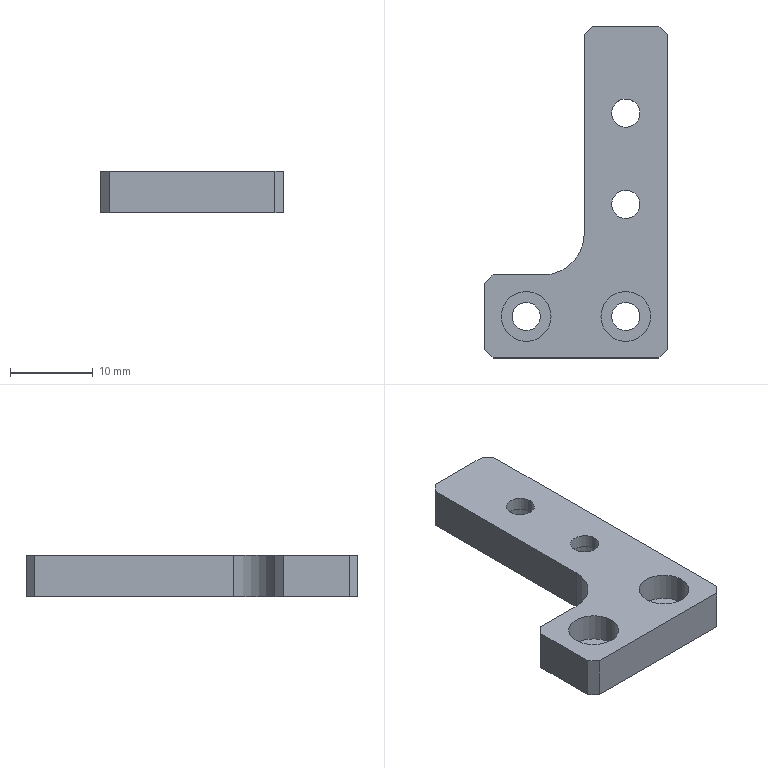Part | STEP file | FBDS-TL-003 | 1 solid | 34 faces | box 22 x 40 x 5 mm | volume 2172 mm3 | cylinder 17 | plane 17 | commonest cylinder face diameters 3.4 x8 6 x8 10 x1
STEP:
#1=CARTESIAN_POINT('',(-3.,-15.,1.6));
#2=VERTEX_POINT('',#1);
#3=CARTESIAN_POINT('',(3.,-15.,1.6));
#4=VERTEX_POINT('',#3);
#5=CARTESIAN_POINT('',(0.,-15.,1.6));
#6=DIRECTION('',(0.,0.,1.));
#7=DIRECTION('',(1.,0.,0.));
#8=AXIS2_PLACEMENT_3D('',#5,#6,#7);
#9=CIRCLE('',#8,3.);
#10=EDGE_CURVE('',#2,#4,#9,.T.);
#11=ORIENTED_EDGE('',*,*,#10,.F.);
#12=CARTESIAN_POINT('',(-3.,-15.,5.));
#13=VERTEX_POINT('',#12);
#14=CARTESIAN_POINT('',(-3.,-15.,5.));
#15=DIRECTION('',(0.,0.,1.));
#16=VECTOR('',#15,1000.);
#17=LINE('',#14,#16);
#18=EDGE_CURVE('',#2,#13,#17,.T.);
#19=ORIENTED_EDGE('',*,*,#18,.T.);
#20=CARTESIAN_POINT('',(3.,-15.,5.));
#21=VERTEX_POINT('',#20);
#22=CARTESIAN_POINT('',(0.,-15.,5.));
#23=DIRECTION('',(0.,0.,1.));
#24=DIRECTION('',(1.,0.,0.));
#25=AXIS2_PLACEMENT_3D('',#22,#23,#24);
#26=CIRCLE('',#25,3.);
#27=EDGE_CURVE('',#13,#21,#26,.T.);
#28=ORIENTED_EDGE('',*,*,#27,.T.);
#29=CARTESIAN_POINT('',(3.,-15.,5.));
#30=DIRECTION('',(0.,0.,1.));
#31=VECTOR('',#30,1000.);
#32=LINE('',#29,#31);
#33=EDGE_CURVE('',#4,#21,#32,.T.);
#34=ORIENTED_EDGE('',*,*,#33,.F.);
#35=EDGE_LOOP('',(#11,#19,#28,#34));
#36=FACE_OUTER_BOUND('',#35,.T.);
#37=CARTESIAN_POINT('',(0.,-15.,5.));
#38=DIRECTION('',(0.,0.,1.));
#39=DIRECTION('',(1.,0.,0.));
#40=AXIS2_PLACEMENT_3D('',#37,#38,#39);
#41=CYLINDRICAL_SURFACE('',#40,3.);
#42=ADVANCED_FACE('',(#36),#41,.F.);
#43=CARTESIAN_POINT('',(1.7,-15.,0.));
#44=VERTEX_POINT('',#43);
#45=CARTESIAN_POINT('',(-1.7,-15.,0.));
#46=VERTEX_POINT('',#45);
#47=CARTESIAN_POINT('',(0.,-15.,0.));
#48=DIRECTION('',(0.,0.,-1.));
#49=DIRECTION('',(-1.,0.,0.));
#50=AXIS2_PLACEMENT_3D('',#47,#48,#49);
#51=CIRCLE('',#50,1.7);
#52=EDGE_CURVE('',#44,#46,#51,.T.);
#53=ORIENTED_EDGE('',*,*,#52,.T.);
#54=CARTESIAN_POINT('',(-1.7,-15.,1.6));
#55=VERTEX_POINT('',#54);
#56=CARTESIAN_POINT('',(-1.7,-15.,5.));
#57=DIRECTION('',(0.,0.,1.));
#58=VECTOR('',#57,1000.);
#59=LINE('',#56,#58);
#60=EDGE_CURVE('',#46,#55,#59,.T.);
#61=ORIENTED_EDGE('',*,*,#60,.T.);
#62=CARTESIAN_POINT('',(1.7,-15.,1.6));
#63=VERTEX_POINT('',#62);
#64=CARTESIAN_POINT('',(0.,-15.,1.6));
#65=DIRECTION('',(0.,0.,1.));
#66=DIRECTION('',(1.,0.,0.));
#67=AXIS2_PLACEMENT_3D('',#64,#65,#66);
#68=CIRCLE('',#67,1.7);
#69=EDGE_CURVE('',#55,#63,#68,.T.);
#70=ORIENTED_EDGE('',*,*,#69,.T.);
#71=CARTESIAN_POINT('',(1.7,-15.,5.));
#72=DIRECTION('',(0.,0.,1.));
#73=VECTOR('',#72,1000.);
#74=LINE('',#71,#73);
#75=EDGE_CURVE('',#44,#63,#74,.T.);
#76=ORIENTED_EDGE('',*,*,#75,.F.);
#77=EDGE_LOOP('',(#53,#61,#70,#76));
#78=FACE_OUTER_BOUND('',#77,.T.);
#79=CARTESIAN_POINT('',(0.,-15.,5.));
#80=DIRECTION('',(0.,0.,1.));
#81=DIRECTION('',(1.,0.,0.));
#82=AXIS2_PLACEMENT_3D('',#79,#80,#81);
#83=CYLINDRICAL_SURFACE('',#82,1.7);
#84=ADVANCED_FACE('',(#78),#83,.F.);
#85=CARTESIAN_POINT('',(-15.,-15.,1.6));
#86=VERTEX_POINT('',#85);
#87=CARTESIAN_POINT('',(-9.,-15.,1.6));
#88=VERTEX_POINT('',#87);
#89=CARTESIAN_POINT('',(-12.,-15.,1.6));
#90=DIRECTION('',(0.,0.,1.));
#91=DIRECTION('',(1.,0.,0.));
#92=AXIS2_PLACEMENT_3D('',#89,#90,#91);
#93=CIRCLE('',#92,3.);
#94=EDGE_CURVE('',#86,#88,#93,.T.);
#95=ORIENTED_EDGE('',*,*,#94,.F.);
#96=CARTESIAN_POINT('',(-15.,-15.,5.));
#97=VERTEX_POINT('',#96);
#98=CARTESIAN_POINT('',(-15.,-15.,5.));
#99=DIRECTION('',(0.,0.,1.));
#100=VECTOR('',#99,1000.);
#101=LINE('',#98,#100);
#102=EDGE_CURVE('',#86,#97,#101,.T.);
#103=ORIENTED_EDGE('',*,*,#102,.T.);
#104=CARTESIAN_POINT('',(-9.,-15.,5.));
#105=VERTEX_POINT('',#104);
#106=CARTESIAN_POINT('',(-12.,-15.,5.));
#107=DIRECTION('',(0.,0.,1.));
#108=DIRECTION('',(1.,0.,0.));
#109=AXIS2_PLACEMENT_3D('',#106,#107,#108);
#110=CIRCLE('',#109,3.);
#111=EDGE_CURVE('',#97,#105,#110,.T.);
#112=ORIENTED_EDGE('',*,*,#111,.T.);
#113=CARTESIAN_POINT('',(-9.,-15.,5.));
#114=DIRECTION('',(0.,0.,1.));
#115=VECTOR('',#114,1000.);
#116=LINE('',#113,#115);
#117=EDGE_CURVE('',#88,#105,#116,.T.);
#118=ORIENTED_EDGE('',*,*,#117,.F.);
#119=EDGE_LOOP('',(#95,#103,#112,#118));
#120=FACE_OUTER_BOUND('',#119,.T.);
#121=CARTESIAN_POINT('',(-12.,-15.,5.));
#122=DIRECTION('',(0.,0.,1.));
#123=DIRECTION('',(1.,0.,0.));
#124=AXIS2_PLACEMENT_3D('',#121,#122,#123);
#125=CYLINDRICAL_SURFACE('',#124,3.);
#126=ADVANCED_FACE('',(#120),#125,.F.);
#127=CARTESIAN_POINT('',(-10.3,-15.,0.));
#128=VERTEX_POINT('',#127);
#129=CARTESIAN_POINT('',(-13.7,-15.,0.));
#130=VERTEX_POINT('',#129);
#131=CARTESIAN_POINT('',(-12.,-15.,0.));
#132=DIRECTION('',(0.,0.,-1.));
#133=DIRECTION('',(-1.,0.,0.));
#134=AXIS2_PLACEMENT_3D('',#131,#132,#133);
#135=CIRCLE('',#134,1.7);
#136=EDGE_CURVE('',#128,#130,#135,.T.);
#137=ORIENTED_EDGE('',*,*,#136,.T.);
#138=CARTESIAN_POINT('',(-13.7,-15.,1.6));
#139=VERTEX_POINT('',#138);
#140=CARTESIAN_POINT('',(-13.7,-15.,5.));
#141=DIRECTION('',(0.,0.,1.));
#142=VECTOR('',#141,1000.);
#143=LINE('',#140,#142);
#144=EDGE_CURVE('',#130,#139,#143,.T.);
#145=ORIENTED_EDGE('',*,*,#144,.T.);
#146=CARTESIAN_POINT('',(-10.3,-15.,1.6));
#147=VERTEX_POINT('',#146);
#148=CARTESIAN_POINT('',(-12.,-15.,1.6));
#149=DIRECTION('',(0.,0.,1.));
#150=DIRECTION('',(1.,0.,0.));
#151=AXIS2_PLACEMENT_3D('',#148,#149,#150);
#152=CIRCLE('',#151,1.7);
#153=EDGE_CURVE('',#139,#147,#152,.T.);
#154=ORIENTED_EDGE('',*,*,#153,.T.);
#155=CARTESIAN_POINT('',(-10.3,-15.,5.));
#156=DIRECTION('',(0.,0.,1.));
#157=VECTOR('',#156,1000.);
#158=LINE('',#155,#157);
#159=EDGE_CURVE('',#128,#147,#158,.T.);
#160=ORIENTED_EDGE('',*,*,#159,.F.);
#161=EDGE_LOOP('',(#137,#145,#154,#160));
#162=FACE_OUTER_BOUND('',#161,.T.);
#163=CARTESIAN_POINT('',(-12.,-15.,5.));
#164=DIRECTION('',(0.,0.,1.));
#165=DIRECTION('',(1.,0.,0.));
#166=AXIS2_PLACEMENT_3D('',#163,#164,#165);
#167=CYLINDRICAL_SURFACE('',#166,1.7);
#168=ADVANCED_FACE('',(#162),#167,.F.);
#169=CARTESIAN_POINT('',(3.,-1.5,3.4));
#170=VERTEX_POINT('',#169);
#171=CARTESIAN_POINT('',(-3.,-1.5,3.4));
#172=VERTEX_POINT('',#171);
#173=CARTESIAN_POINT('',(0.,-1.5,3.4));
#174=DIRECTION('',(0.,0.,-1.));
#175=DIRECTION('',(-1.,0.,0.));
#176=AXIS2_PLACEMENT_3D('',#173,#174,#175);
#177=CIRCLE('',#176,3.);
#178=EDGE_CURVE('',#170,#172,#177,.T.);
#179=ORIENTED_EDGE('',*,*,#178,.F.);
#180=CARTESIAN_POINT('',(3.,-1.5,0.));
#181=VERTEX_POINT('',#180);
#182=CARTESIAN_POINT('',(3.,-1.5,0.));
#183=DIRECTION('',(0.,0.,-1.));
#184=VECTOR('',#183,1000.);
#185=LINE('',#182,#184);
#186=EDGE_CURVE('',#170,#181,#185,.T.);
#187=ORIENTED_EDGE('',*,*,#186,.T.);
#188=CARTESIAN_POINT('',(-3.,-1.5,0.));
#189=VERTEX_POINT('',#188);
#190=CARTESIAN_POINT('',(0.,-1.5,0.));
#191=DIRECTION('',(0.,0.,-1.));
#192=DIRECTION('',(-1.,0.,0.));
#193=AXIS2_PLACEMENT_3D('',#190,#191,#192);
#194=CIRCLE('',#193,3.);
#195=EDGE_CURVE('',#181,#189,#194,.T.);
#196=ORIENTED_EDGE('',*,*,#195,.T.);
#197=CARTESIAN_POINT('',(-3.,-1.5,0.));
#198=DIRECTION('',(0.,0.,-1.));
#199=VECTOR('',#198,1000.);
#200=LINE('',#197,#199);
#201=EDGE_CURVE('',#172,#189,#200,.T.);
#202=ORIENTED_EDGE('',*,*,#201,.F.);
#203=EDGE_LOOP('',(#179,#187,#196,#202));
#204=FACE_OUTER_BOUND('',#203,.T.);
#205=CARTESIAN_POINT('',(0.,-1.5,0.));
#206=DIRECTION('',(0.,0.,-1.));
#207=DIRECTION('',(-1.,0.,0.));
#208=AXIS2_PLACEMENT_3D('',#205,#206,#207);
#209=CYLINDRICAL_SURFACE('',#208,3.);
#210=ADVANCED_FACE('',(#204),#209,.F.);
#211=CARTESIAN_POINT('',(1.7,-1.5,5.));
#212=VERTEX_POINT('',#211);
#213=CARTESIAN_POINT('',(-1.7,-1.5,5.));
#214=VERTEX_POINT('',#213);
#215=CARTESIAN_POINT('',(0.,-1.5,5.));
#216=DIRECTION('',(0.,0.,-1.));
#217=DIRECTION('',(-1.,0.,0.));
#218=AXIS2_PLACEMENT_3D('',#215,#216,#217);
#219=CIRCLE('',#218,1.7);
#220=EDGE_CURVE('',#212,#214,#219,.T.);
#221=ORIENTED_EDGE('',*,*,#220,.F.);
#222=CARTESIAN_POINT('',(1.7,-1.5,3.4));
#223=VERTEX_POINT('',#222);
#224=CARTESIAN_POINT('',(1.7,-1.5,0.));
#225=DIRECTION('',(0.,0.,-1.));
#226=VECTOR('',#225,1000.);
#227=LINE('',#224,#226);
#228=EDGE_CURVE('',#212,#223,#227,.T.);
#229=ORIENTED_EDGE('',*,*,#228,.T.);
#230=CARTESIAN_POINT('',(-1.7,-1.5,3.4));
#231=VERTEX_POINT('',#230);
#232=CARTESIAN_POINT('',(0.,-1.5,3.4));
#233=DIRECTION('',(0.,0.,-1.));
#234=DIRECTION('',(-1.,0.,0.));
#235=AXIS2_PLACEMENT_3D('',#232,#233,#234);
#236=CIRCLE('',#235,1.7);
#237=EDGE_CURVE('',#223,#231,#236,.T.);
#238=ORIENTED_EDGE('',*,*,#237,.T.);
#239=CARTESIAN_POINT('',(-1.7,-1.5,0.));
#240=DIRECTION('',(0.,0.,-1.));
#241=VECTOR('',#240,1000.);
#242=LINE('',#239,#241);
#243=EDGE_CURVE('',#214,#231,#242,.T.);
#244=ORIENTED_EDGE('',*,*,#243,.F.);
#245=EDGE_LOOP('',(#221,#229,#238,#244));
#246=FACE_OUTER_BOUND('',#245,.T.);
#247=CARTESIAN_POINT('',(0.,-1.5,0.));
#248=DIRECTION('',(0.,0.,-1.));
#249=DIRECTION('',(-1.,0.,0.));
#250=AXIS2_PLACEMENT_3D('',#247,#248,#249);
#251=CYLINDRICAL_SURFACE('',#250,1.7);
#252=ADVANCED_FACE('',(#246),#251,.F.);
#253=CARTESIAN_POINT('',(3.,9.5,3.4));
#254=VERTEX_POINT('',#253);
#255=CARTESIAN_POINT('',(-3.,9.5,3.4));
#256=VERTEX_POINT('',#255);
#257=CARTESIAN_POINT('',(0.,9.5,3.4));
#258=DIRECTION('',(0.,0.,-1.));
#259=DIRECTION('',(-1.,0.,0.));
#260=AXIS2_PLACEMENT_3D('',#257,#258,#259);
#261=CIRCLE('',#260,3.);
#262=EDGE_CURVE('',#254,#256,#261,.T.);
#263=ORIENTED_EDGE('',*,*,#262,.F.);
#264=CARTESIAN_POINT('',(3.,9.5,0.));
#265=VERTEX_POINT('',#264);
#266=CARTESIAN_POINT('',(3.,9.5,0.));
#267=DIRECTION('',(0.,0.,-1.));
#268=VECTOR('',#267,1000.);
#269=LINE('',#266,#268);
#270=EDGE_CURVE('',#254,#265,#269,.T.);
#271=ORIENTED_EDGE('',*,*,#270,.T.);
#272=CARTESIAN_POINT('',(-3.,9.5,0.));
#273=VERTEX_POINT('',#272);
#274=CARTESIAN_POINT('',(0.,9.5,0.));
#275=DIRECTION('',(0.,0.,-1.));
#276=DIRECTION('',(-1.,0.,0.));
#277=AXIS2_PLACEMENT_3D('',#274,#275,#276);
#278=CIRCLE('',#277,3.);
#279=EDGE_CURVE('',#265,#273,#278,.T.);
#280=ORIENTED_EDGE('',*,*,#279,.T.);
#281=CARTESIAN_POINT('',(-3.,9.5,0.));
#282=DIRECTION('',(0.,0.,-1.));
#283=VECTOR('',#282,1000.);
#284=LINE('',#281,#283);
#285=EDGE_CURVE('',#256,#273,#284,.T.);
#286=ORIENTED_EDGE('',*,*,#285,.F.);
#287=EDGE_LOOP('',(#263,#271,#280,#286));
#288=FACE_OUTER_BOUND('',#287,.T.);
#289=CARTESIAN_POINT('',(0.,9.5,0.));
#290=DIRECTION('',(0.,0.,-1.));
#291=DIRECTION('',(-1.,0.,0.));
#292=AXIS2_PLACEMENT_3D('',#289,#290,#291);
#293=CYLINDRICAL_SURFACE('',#292,3.);
#294=ADVANCED_FACE('',(#288),#293,.F.);
#295=CARTESIAN_POINT('',(1.7,9.5,5.));
#296=VERTEX_POINT('',#295);
#297=CARTESIAN_POINT('',(-1.7,9.5,5.));
#298=VERTEX_POINT('',#297);
#299=CARTESIAN_POINT('',(0.,9.5,5.));
#300=DIRECTION('',(0.,0.,-1.));
#301=DIRECTION('',(-1.,0.,0.));
#302=AXIS2_PLACEMENT_3D('',#299,#300,#301);
#303=CIRCLE('',#302,1.7);
#304=EDGE_CURVE('',#296,#298,#303,.T.);
#305=ORIENTED_EDGE('',*,*,#304,.F.);
#306=CARTESIAN_POINT('',(1.7,9.5,3.4));
#307=VERTEX_POINT('',#306);
#308=CARTESIAN_POINT('',(1.7,9.5,0.));
#309=DIRECTION('',(0.,0.,-1.));
#310=VECTOR('',#309,1000.);
#311=LINE('',#308,#310);
#312=EDGE_CURVE('',#296,#307,#311,.T.);
#313=ORIENTED_EDGE('',*,*,#312,.T.);
#314=CARTESIAN_POINT('',(-1.7,9.5,3.4));
#315=VERTEX_POINT('',#314);
#316=CARTESIAN_POINT('',(0.,9.5,3.4));
#317=DIRECTION('',(0.,0.,-1.));
#318=DIRECTION('',(-1.,0.,0.));
#319=AXIS2_PLACEMENT_3D('',#316,#317,#318);
#320=CIRCLE('',#319,1.7);
#321=EDGE_CURVE('',#307,#315,#320,.T.);
#322=ORIENTED_EDGE('',*,*,#321,.T.);
#323=CARTESIAN_POINT('',(-1.7,9.5,0.));
#324=DIRECTION('',(0.,0.,-1.));
#325=VECTOR('',#324,1000.);
#326=LINE('',#323,#325);
#327=EDGE_CURVE('',#298,#315,#326,.T.);
#328=ORIENTED_EDGE('',*,*,#327,.F.);
#329=EDGE_LOOP('',(#305,#313,#322,#328));
#330=FACE_OUTER_BOUND('',#329,.T.);
#331=CARTESIAN_POINT('',(0.,9.5,0.));
#332=DIRECTION('',(0.,0.,-1.));
#333=DIRECTION('',(-1.,0.,0.));
#334=AXIS2_PLACEMENT_3D('',#331,#332,#333);
#335=CYLINDRICAL_SURFACE('',#334,1.7);
#336=ADVANCED_FACE('',(#330),#335,.F.);
#337=CARTESIAN_POINT('',(5.,-19.,0.));
#338=VERTEX_POINT('',#337);
#339=CARTESIAN_POINT('',(5.,19.,0.));
#340=VERTEX_POINT('',#339);
#341=CARTESIAN_POINT('',(5.,-20.,0.));
#342=DIRECTION('',(0.,1.,0.));
#343=VECTOR('',#342,1000.);
#344=LINE('',#341,#343);
#345=EDGE_CURVE('',#338,#340,#344,.T.);
#346=ORIENTED_EDGE('',*,*,#345,.T.);
#347=CARTESIAN_POINT('',(5.,19.,5.));
#348=VERTEX_POINT('',#347);
#349=CARTESIAN_POINT('',(5.,19.,5.));
#350=DIRECTION('',(0.,0.,1.));
#351=VECTOR('',#350,1000.);
#352=LINE('',#349,#351);
#353=EDGE_CURVE('',#340,#348,#352,.T.);
#354=ORIENTED_EDGE('',*,*,#353,.T.);
#355=CARTESIAN_POINT('',(5.,-19.,5.));
#356=VERTEX_POINT('',#355);
#357=CARTESIAN_POINT('',(5.,-20.,5.));
#358=DIRECTION('',(0.,1.,0.));
#359=VECTOR('',#358,1000.);
#360=LINE('',#357,#359);
#361=EDGE_CURVE('',#356,#348,#360,.T.);
#362=ORIENTED_EDGE('',*,*,#361,.F.);
#363=CARTESIAN_POINT('',(5.,-19.,5.));
#364=DIRECTION('',(0.,0.,-1.));
#365=VECTOR('',#364,1000.);
#366=LINE('',#363,#365);
#367=EDGE_CURVE('',#356,#338,#366,.T.);
#368=ORIENTED_EDGE('',*,*,#367,.T.);
#369=EDGE_LOOP('',(#346,#354,#362,#368));
#370=FACE_OUTER_BOUND('',#369,.T.);
#371=CARTESIAN_POINT('',(5.,-20.,5.));
#372=DIRECTION('',(-1.,0.,0.));
#373=DIRECTION('',(0.,0.,1.));
#374=AXIS2_PLACEMENT_3D('',#371,#372,#373);
#375=PLANE('',#374);
#376=ADVANCED_FACE('',(#370),#375,.F.);
#377=CARTESIAN_POINT('',(4.,20.,5.));
#378=VERTEX_POINT('',#377);
#379=CARTESIAN_POINT('',(-4.,20.,5.));
#380=VERTEX_POINT('',#379);
#381=CARTESIAN_POINT('',(-5.,20.,5.));
#382=DIRECTION('',(-1.,0.,0.));
#383=VECTOR('',#382,1000.);
#384=LINE('',#381,#383);
#385=EDGE_CURVE('',#378,#380,#384,.T.);
#386=ORIENTED_EDGE('',*,*,#385,.F.);
#387=CARTESIAN_POINT('',(4.,20.,0.));
#388=VERTEX_POINT('',#387);
#389=CARTESIAN_POINT('',(4.,20.,5.));
#390=DIRECTION('',(0.,0.,-1.));
#391=VECTOR('',#390,1000.);
#392=LINE('',#389,#391);
#393=EDGE_CURVE('',#378,#388,#392,.T.);
#394=ORIENTED_EDGE('',*,*,#393,.T.);
#395=CARTESIAN_POINT('',(-4.,20.,0.));
#396=VERTEX_POINT('',#395);
#397=CARTESIAN_POINT('',(-5.,20.,0.));
#398=DIRECTION('',(-1.,0.,0.));
#399=VECTOR('',#398,1000.);
#400=LINE('',#397,#399);
#401=EDGE_CURVE('',#388,#396,#400,.T.);
#402=ORIENTED_EDGE('',*,*,#401,.T.);
#403=CARTESIAN_POINT('',(-4.,20.,5.));
#404=DIRECTION('',(0.,0.,1.));
#405=VECTOR('',#404,1000.);
#406=LINE('',#403,#405);
#407=EDGE_CURVE('',#396,#380,#406,.T.);
#408=ORIENTED_EDGE('',*,*,#407,.T.);
#409=EDGE_LOOP('',(#386,#394,#402,#408));
#410=FACE_OUTER_BOUND('',#409,.T.);
#411=CARTESIAN_POINT('',(-5.,20.,5.));
#412=DIRECTION('',(0.,-1.,0.));
#413=DIRECTION('',(0.,0.,-1.));
#414=AXIS2_PLACEMENT_3D('',#411,#412,#413);
#415=PLANE('',#414);
#416=ADVANCED_FACE('',(#410),#415,.F.);
#417=CARTESIAN_POINT('',(-5.,19.,5.));
#418=VERTEX_POINT('',#417);
#419=CARTESIAN_POINT('',(-5.,-5.,5.));
#420=VERTEX_POINT('',#419);
#421=CARTESIAN_POINT('',(-5.,-20.,5.));
#422=DIRECTION('',(0.,-1.,0.));
#423=VECTOR('',#422,1000.);
#424=LINE('',#421,#423);
#425=EDGE_CURVE('',#418,#420,#424,.T.);
#426=ORIENTED_EDGE('',*,*,#425,.F.);
#427=CARTESIAN_POINT('',(-5.,19.,0.));
#428=VERTEX_POINT('',#427);
#429=CARTESIAN_POINT('',(-5.,19.,5.));
#430=DIRECTION('',(0.,0.,-1.));
#431=VECTOR('',#430,1000.);
#432=LINE('',#429,#431);
#433=EDGE_CURVE('',#418,#428,#432,.T.);
#434=ORIENTED_EDGE('',*,*,#433,.T.);
#435=CARTESIAN_POINT('',(-5.,-5.,0.));
#436=VERTEX_POINT('',#435);
#437=CARTESIAN_POINT('',(-5.,-20.,0.));
#438=DIRECTION('',(0.,-1.,0.));
#439=VECTOR('',#438,1000.);
#440=LINE('',#437,#439);
#441=EDGE_CURVE('',#428,#436,#440,.T.);
#442=ORIENTED_EDGE('',*,*,#441,.T.);
#443=CARTESIAN_POINT('',(-5.,-5.,5.));
#444=DIRECTION('',(0.,0.,1.));
#445=VECTOR('',#444,1000.);
#446=LINE('',#443,#445);
#447=EDGE_CURVE('',#436,#420,#446,.T.);
#448=ORIENTED_EDGE('',*,*,#447,.T.);
#449=EDGE_LOOP('',(#426,#434,#442,#448));
#450=FACE_OUTER_BOUND('',#449,.T.);
#451=CARTESIAN_POINT('',(-5.,-20.,5.));
#452=DIRECTION('',(1.,0.,0.));
#453=DIRECTION('',(0.,0.,-1.));
#454=AXIS2_PLACEMENT_3D('',#451,#452,#453);
#455=PLANE('',#454);
#456=ADVANCED_FACE('',(#450),#455,.F.);
#457=CARTESIAN_POINT('',(-16.,-20.,5.));
#458=VERTEX_POINT('',#457);
#459=CARTESIAN_POINT('',(4.,-20.,5.));
#460=VERTEX_POINT('',#459);
#461=CARTESIAN_POINT('',(-5.,-20.,5.));
#462=DIRECTION('',(1.,0.,0.));
#463=VECTOR('',#462,1000.);
#464=LINE('',#461,#463);
#465=EDGE_CURVE('',#458,#460,#464,.T.);
#466=ORIENTED_EDGE('',*,*,#465,.F.);
#467=CARTESIAN_POINT('',(-16.,-20.,0.));
#468=VERTEX_POINT('',#467);
#469=CARTESIAN_POINT('',(-16.,-20.,0.));
#470=DIRECTION('',(0.,0.,-1.));
#471=VECTOR('',#470,1000.);
#472=LINE('',#469,#471);
#473=EDGE_CURVE('',#458,#468,#472,.T.);
#474=ORIENTED_EDGE('',*,*,#473,.T.);
#475=CARTESIAN_POINT('',(4.,-20.,0.));
#476=VERTEX_POINT('',#475);
#477=CARTESIAN_POINT('',(-5.,-20.,0.));
#478=DIRECTION('',(1.,0.,0.));
#479=VECTOR('',#478,1000.);
#480=LINE('',#477,#479);
#481=EDGE_CURVE('',#468,#476,#480,.T.);
#482=ORIENTED_EDGE('',*,*,#481,.T.);
#483=CARTESIAN_POINT('',(4.,-20.,5.));
#484=DIRECTION('',(0.,0.,1.));
#485=VECTOR('',#484,1000.);
#486=LINE('',#483,#485);
#487=EDGE_CURVE('',#476,#460,#486,.T.);
#488=ORIENTED_EDGE('',*,*,#487,.T.);
#489=EDGE_LOOP('',(#466,#474,#482,#488));
#490=FACE_OUTER_BOUND('',#489,.T.);
#491=CARTESIAN_POINT('',(-5.,-20.,5.));
#492=DIRECTION('',(0.,1.,0.));
#493=DIRECTION('',(0.,0.,1.));
#494=AXIS2_PLACEMENT_3D('',#491,#492,#493);
#495=PLANE('',#494);
#496=ADVANCED_FACE('',(#490),#495,.F.);
#497=CARTESIAN_POINT('',(0.,-15.,5.));
#498=DIRECTION('',(0.,0.,1.));
#499=DIRECTION('',(1.,0.,0.));
#500=AXIS2_PLACEMENT_3D('',#497,#498,#499);
#501=CIRCLE('',#500,3.);
#502=EDGE_CURVE('',#21,#13,#501,.T.);
#503=ORIENTED_EDGE('',*,*,#502,.F.);
#504=ORIENTED_EDGE('',*,*,#27,.F.);
#505=EDGE_LOOP('',(#503,#504));
#506=FACE_BOUND('',#505,.T.);
#507=CARTESIAN_POINT('',(-12.,-15.,5.));
#508=DIRECTION('',(0.,0.,1.));
#509=DIRECTION('',(1.,0.,0.));
#510=AXIS2_PLACEMENT_3D('',#507,#508,#509);
#511=CIRCLE('',#510,3.);
#512=EDGE_CURVE('',#105,#97,#511,.T.);
#513=ORIENTED_EDGE('',*,*,#512,.F.);
#514=ORIENTED_EDGE('',*,*,#111,.F.);
#515=EDGE_LOOP('',(#513,#514));
#516=FACE_BOUND('',#515,.T.);
#517=CARTESIAN_POINT('',(0.,-1.5,5.));
#518=DIRECTION('',(0.,0.,-1.));
#519=DIRECTION('',(-1.,0.,0.));
#520=AXIS2_PLACEMENT_3D('',#517,#518,#519);
#521=CIRCLE('',#520,1.7);
#522=EDGE_CURVE('',#214,#212,#521,.T.);
#523=ORIENTED_EDGE('',*,*,#522,.T.);
#524=ORIENTED_EDGE('',*,*,#220,.T.);
#525=EDGE_LOOP('',(#523,#524));
#526=FACE_BOUND('',#525,.T.);
#527=CARTESIAN_POINT('',(0.,9.5,5.));
#528=DIRECTION('',(0.,0.,-1.));
#529=DIRECTION('',(-1.,0.,0.));
#530=AXIS2_PLACEMENT_3D('',#527,#528,#529);
#531=CIRCLE('',#530,1.7);
#532=EDGE_CURVE('',#298,#296,#531,.T.);
#533=ORIENTED_EDGE('',*,*,#532,.T.);
#534=ORIENTED_EDGE('',*,*,#304,.T.);
#535=EDGE_LOOP('',(#533,#534));
#536=FACE_BOUND('',#535,.T.);
#537=ORIENTED_EDGE('',*,*,#361,.T.);
#538=CARTESIAN_POINT('',(4.,20.,5.));
#539=DIRECTION('',(-0.7071,0.7071,0.));
#540=VECTOR('',#539,1000.);
#541=LINE('',#538,#540);
#542=EDGE_CURVE('',#348,#378,#541,.T.);
#543=ORIENTED_EDGE('',*,*,#542,.T.);
#544=ORIENTED_EDGE('',*,*,#385,.T.);
#545=CARTESIAN_POINT('',(-5.,19.,5.));
#546=DIRECTION('',(-0.7071,-0.7071,0.));
#547=VECTOR('',#546,1000.);
#548=LINE('',#545,#547);
#549=EDGE_CURVE('',#380,#418,#548,.T.);
#550=ORIENTED_EDGE('',*,*,#549,.T.);
#551=ORIENTED_EDGE('',*,*,#425,.T.);
#552=CARTESIAN_POINT('',(-10.,-10.,5.));
#553=VERTEX_POINT('',#552);
#554=CARTESIAN_POINT('',(-10.,-5.,5.));
#555=DIRECTION('',(0.,0.,-1.));
#556=DIRECTION('',(-1.,0.,0.));
#557=AXIS2_PLACEMENT_3D('',#554,#555,#556);
#558=CIRCLE('',#557,5.);
#559=EDGE_CURVE('',#420,#553,#558,.T.);
#560=ORIENTED_EDGE('',*,*,#559,.T.);
#561=CARTESIAN_POINT('',(-16.,-10.,5.));
#562=VERTEX_POINT('',#561);
#563=CARTESIAN_POINT('',(-5.,-10.,5.));
#564=DIRECTION('',(-1.,0.,0.));
#565=VECTOR('',#564,1000.);
#566=LINE('',#563,#565);
#567=EDGE_CURVE('',#553,#562,#566,.T.);
#568=ORIENTED_EDGE('',*,*,#567,.T.);
#569=CARTESIAN_POINT('',(-17.,-11.,5.));
#570=VERTEX_POINT('',#569);
#571=CARTESIAN_POINT('',(-16.,-10.,5.));
#572=DIRECTION('',(-0.7071,-0.7071,0.));
#573=VECTOR('',#572,1000.);
#574=LINE('',#571,#573);
#575=EDGE_CURVE('',#562,#570,#574,.T.);
#576=ORIENTED_EDGE('',*,*,#575,.T.);
#577=CARTESIAN_POINT('',(-17.,-19.,5.));
#578=VERTEX_POINT('',#577);
#579=CARTESIAN_POINT('',(-17.,-20.,5.));
#580=DIRECTION('',(0.,-1.,0.));
#581=VECTOR('',#580,1000.);
#582=LINE('',#579,#581);
#583=EDGE_CURVE('',#570,#578,#582,.T.);
#584=ORIENTED_EDGE('',*,*,#583,.T.);
#585=CARTESIAN_POINT('',(-17.,-19.,5.));
#586=DIRECTION('',(0.7071,-0.7071,0.));
#587=VECTOR('',#586,1000.);
#588=LINE('',#585,#587);
#589=EDGE_CURVE('',#578,#458,#588,.T.);
#590=ORIENTED_EDGE('',*,*,#589,.T.);
#591=ORIENTED_EDGE('',*,*,#465,.T.);
#592=CARTESIAN_POINT('',(5.,-19.,5.));
#593=DIRECTION('',(0.7071,0.7071,0.));
#594=VECTOR('',#593,1000.);
#595=LINE('',#592,#594);
#596=EDGE_CURVE('',#460,#356,#595,.T.);
#597=ORIENTED_EDGE('',*,*,#596,.T.);
#598=EDGE_LOOP('',(#537,#543,#544,#550,#551,#560,#568,#576,#584,#590,#591,#597));
#599=FACE_OUTER_BOUND('',#598,.T.);
#600=CARTESIAN_POINT('',(0.,0.,5.));
#601=DIRECTION('',(0.,0.,-1.));
#602=DIRECTION('',(-1.,0.,0.));
#603=AXIS2_PLACEMENT_3D('',#600,#601,#602);
#604=PLANE('',#603);
#605=ADVANCED_FACE('',(#506,#516,#526,#536,#599),#604,.F.);
#606=ORIENTED_EDGE('',*,*,#52,.F.);
#607=CARTESIAN_POINT('',(0.,-15.,0.));
#608=DIRECTION('',(0.,0.,-1.));
#609=DIRECTION('',(-1.,0.,0.));
#610=AXIS2_PLACEMENT_3D('',#607,#608,#609);
#611=CIRCLE('',#610,1.7);
#612=EDGE_CURVE('',#46,#44,#611,.T.);
#613=ORIENTED_EDGE('',*,*,#612,.F.);
#614=EDGE_LOOP('',(#606,#613));
#615=FACE_BOUND('',#614,.T.);
#616=ORIENTED_EDGE('',*,*,#136,.F.);
#617=CARTESIAN_POINT('',(-12.,-15.,0.));
#618=DIRECTION('',(0.,0.,-1.));
#619=DIRECTION('',(-1.,0.,0.));
#620=AXIS2_PLACEMENT_3D('',#617,#618,#619);
#621=CIRCLE('',#620,1.7);
#622=EDGE_CURVE('',#130,#128,#621,.T.);
#623=ORIENTED_EDGE('',*,*,#622,.F.);
#624=EDGE_LOOP('',(#616,#623));
#625=FACE_BOUND('',#624,.T.);
#626=CARTESIAN_POINT('',(0.,-1.5,0.));
#627=DIRECTION('',(0.,0.,-1.));
#628=DIRECTION('',(-1.,0.,0.));
#629=AXIS2_PLACEMENT_3D('',#626,#627,#628);
#630=CIRCLE('',#629,3.);
#631=EDGE_CURVE('',#189,#181,#630,.T.);
#632=ORIENTED_EDGE('',*,*,#631,.F.);
#633=ORIENTED_EDGE('',*,*,#195,.F.);
#634=EDGE_LOOP('',(#632,#633));
#635=FACE_BOUND('',#634,.T.);
#636=CARTESIAN_POINT('',(0.,9.5,0.));
#637=DIRECTION('',(0.,0.,-1.));
#638=DIRECTION('',(-1.,0.,0.));
#639=AXIS2_PLACEMENT_3D('',#636,#637,#638);
#640=CIRCLE('',#639,3.);
#641=EDGE_CURVE('',#273,#265,#640,.T.);
#642=ORIENTED_EDGE('',*,*,#641,.F.);
#643=ORIENTED_EDGE('',*,*,#279,.F.);
#644=EDGE_LOOP('',(#642,#643));
#645=FACE_BOUND('',#644,.T.);
#646=ORIENTED_EDGE('',*,*,#401,.F.);
#647=CARTESIAN_POINT('',(12.,12.,0.));
#648=DIRECTION('',(0.7071,-0.7071,0.));
#649=VECTOR('',#648,1000.);
#650=LINE('',#647,#649);
#651=EDGE_CURVE('',#388,#340,#650,.T.);
#652=ORIENTED_EDGE('',*,*,#651,.T.);
#653=ORIENTED_EDGE('',*,*,#345,.F.);
#654=CARTESIAN_POINT('',(12.,-12.,0.));
#655=DIRECTION('',(-0.7071,-0.7071,0.));
#656=VECTOR('',#655,1000.);
#657=LINE('',#654,#656);
#658=EDGE_CURVE('',#338,#476,#657,.T.);
#659=ORIENTED_EDGE('',*,*,#658,.T.);
#660=ORIENTED_EDGE('',*,*,#481,.F.);
#661=CARTESIAN_POINT('',(-17.,-19.,0.));
#662=VERTEX_POINT('',#661);
#663=CARTESIAN_POINT('',(-18.,-18.,0.));
#664=DIRECTION('',(-0.7071,0.7071,0.));
#665=VECTOR('',#664,1000.);
#666=LINE('',#663,#665);
#667=EDGE_CURVE('',#468,#662,#666,.T.);
#668=ORIENTED_EDGE('',*,*,#667,.T.);
#669=CARTESIAN_POINT('',(-17.,-11.,0.));
#670=VERTEX_POINT('',#669);
#671=CARTESIAN_POINT('',(-17.,-20.,0.));
#672=DIRECTION('',(0.,-1.,0.));
#673=VECTOR('',#672,1000.);
#674=LINE('',#671,#673);
#675=EDGE_CURVE('',#670,#662,#674,.T.);
#676=ORIENTED_EDGE('',*,*,#675,.F.);
#677=CARTESIAN_POINT('',(-16.,-10.,0.));
#678=VERTEX_POINT('',#677);
#679=CARTESIAN_POINT('',(-3.,3.,0.));
#680=DIRECTION('',(0.7071,0.7071,0.));
#681=VECTOR('',#680,1000.);
#682=LINE('',#679,#681);
#683=EDGE_CURVE('',#670,#678,#682,.T.);
#684=ORIENTED_EDGE('',*,*,#683,.T.);
#685=CARTESIAN_POINT('',(-10.,-10.,0.));
#686=VERTEX_POINT('',#685);
#687=CARTESIAN_POINT('',(-5.,-10.,0.));
#688=DIRECTION('',(-1.,0.,0.));
#689=VECTOR('',#688,1000.);
#690=LINE('',#687,#689);
#691=EDGE_CURVE('',#686,#678,#690,.T.);
#692=ORIENTED_EDGE('',*,*,#691,.F.);
#693=CARTESIAN_POINT('',(-10.,-5.,0.));
#694=DIRECTION('',(0.,0.,1.));
#695=DIRECTION('',(-1.,0.,0.));
#696=AXIS2_PLACEMENT_3D('',#693,#694,#695);
#697=CIRCLE('',#696,5.);
#698=EDGE_CURVE('',#686,#436,#697,.T.);
#699=ORIENTED_EDGE('',*,*,#698,.T.);
#700=ORIENTED_EDGE('',*,*,#441,.F.);
#701=CARTESIAN_POINT('',(-12.,12.,0.));
#702=DIRECTION('',(0.7071,0.7071,0.));
#703=VECTOR('',#702,1000.);
#704=LINE('',#701,#703);
#705=EDGE_CURVE('',#428,#396,#704,.T.);
#706=ORIENTED_EDGE('',*,*,#705,.T.);
#707=EDGE_LOOP('',(#646,#652,#653,#659,#660,#668,#676,#684,#692,#699,#700,#706));
#708=FACE_OUTER_BOUND('',#707,.T.);
#709=CARTESIAN_POINT('',(0.,0.,0.));
#710=DIRECTION('',(0.,0.,-1.));
#711=DIRECTION('',(-1.,0.,0.));
#712=AXIS2_PLACEMENT_3D('',#709,#710,#711);
#713=PLANE('',#712);
#714=ADVANCED_FACE('',(#615,#625,#635,#645,#708),#713,.T.);
#715=ORIENTED_EDGE('',*,*,#691,.T.);
#716=CARTESIAN_POINT('',(-16.,-10.,-15.62));
#717=DIRECTION('',(0.,0.,1.));
#718=VECTOR('',#717,1000.);
#719=LINE('',#716,#718);
#720=EDGE_CURVE('',#678,#562,#719,.T.);
#721=ORIENTED_EDGE('',*,*,#720,.T.);
#722=ORIENTED_EDGE('',*,*,#567,.F.);
#723=CARTESIAN_POINT('',(-10.,-10.,-15.62));
#724=DIRECTION('',(0.,0.,-1.));
#725=VECTOR('',#724,1000.);
#726=LINE('',#723,#725);
#727=EDGE_CURVE('',#553,#686,#726,.T.);
#728=ORIENTED_EDGE('',*,*,#727,.T.);
#729=EDGE_LOOP('',(#715,#721,#722,#728));
#730=FACE_OUTER_BOUND('',#729,.T.);
#731=CARTESIAN_POINT('',(-5.,-10.,-15.62));
#732=DIRECTION('',(0.,1.,0.));
#733=DIRECTION('',(-1.,0.,0.));
#734=AXIS2_PLACEMENT_3D('',#731,#732,#733);
#735=PLANE('',#734);
#736=ADVANCED_FACE('',(#730),#735,.T.);
#737=ORIENTED_EDGE('',*,*,#583,.F.);
#738=CARTESIAN_POINT('',(-17.,-11.,-15.62));
#739=DIRECTION('',(0.,0.,-1.));
#740=VECTOR('',#739,1000.);
#741=LINE('',#738,#740);
#742=EDGE_CURVE('',#570,#670,#741,.T.);
#743=ORIENTED_EDGE('',*,*,#742,.T.);
#744=ORIENTED_EDGE('',*,*,#675,.T.);
#745=CARTESIAN_POINT('',(-17.,-19.,5.));
#746=DIRECTION('',(0.,0.,1.));
#747=VECTOR('',#746,1000.);
#748=LINE('',#745,#747);
#749=EDGE_CURVE('',#662,#578,#748,.T.);
#750=ORIENTED_EDGE('',*,*,#749,.T.);
#751=EDGE_LOOP('',(#737,#743,#744,#750));
#752=FACE_OUTER_BOUND('',#751,.T.);
#753=CARTESIAN_POINT('',(-17.,-20.,-15.62));
#754=DIRECTION('',(-1.,0.,0.));
#755=DIRECTION('',(0.,0.,1.));
#756=AXIS2_PLACEMENT_3D('',#753,#754,#755);
#757=PLANE('',#756);
#758=ADVANCED_FACE('',(#752),#757,.T.);
#759=ORIENTED_EDGE('',*,*,#312,.F.);
#760=ORIENTED_EDGE('',*,*,#532,.F.);
#761=ORIENTED_EDGE('',*,*,#327,.T.);
#762=CARTESIAN_POINT('',(0.,9.5,3.4));
#763=DIRECTION('',(0.,0.,-1.));
#764=DIRECTION('',(-1.,0.,0.));
#765=AXIS2_PLACEMENT_3D('',#762,#763,#764);
#766=CIRCLE('',#765,1.7);
#767=EDGE_CURVE('',#315,#307,#766,.T.);
#768=ORIENTED_EDGE('',*,*,#767,.T.);
#769=EDGE_LOOP('',(#759,#760,#761,#768));
#770=FACE_OUTER_BOUND('',#769,.T.);
#771=CARTESIAN_POINT('',(0.,9.5,0.));
#772=DIRECTION('',(0.,0.,-1.));
#773=DIRECTION('',(-1.,0.,0.));
#774=AXIS2_PLACEMENT_3D('',#771,#772,#773);
#775=CYLINDRICAL_SURFACE('',#774,1.7);
#776=ADVANCED_FACE('',(#770),#775,.F.);
#777=ORIENTED_EDGE('',*,*,#767,.F.);
#778=ORIENTED_EDGE('',*,*,#321,.F.);
#779=EDGE_LOOP('',(#777,#778));
#780=FACE_BOUND('',#779,.T.);
#781=CARTESIAN_POINT('',(0.,9.5,3.4));
#782=DIRECTION('',(0.,0.,-1.));
#783=DIRECTION('',(-1.,0.,0.));
#784=AXIS2_PLACEMENT_3D('',#781,#782,#783);
#785=CIRCLE('',#784,3.);
#786=EDGE_CURVE('',#256,#254,#785,.T.);
#787=ORIENTED_EDGE('',*,*,#786,.T.);
#788=ORIENTED_EDGE('',*,*,#262,.T.);
#789=EDGE_LOOP('',(#787,#788));
#790=FACE_OUTER_BOUND('',#789,.T.);
#791=CARTESIAN_POINT('',(1.7,9.5,3.4));
#792=DIRECTION('',(0.,0.,1.));
#793=DIRECTION('',(1.,0.,0.));
#794=AXIS2_PLACEMENT_3D('',#791,#792,#793);
#795=PLANE('',#794);
#796=ADVANCED_FACE('',(#780,#790),#795,.F.);
#797=ORIENTED_EDGE('',*,*,#270,.F.);
#798=ORIENTED_EDGE('',*,*,#786,.F.);
#799=ORIENTED_EDGE('',*,*,#285,.T.);
#800=ORIENTED_EDGE('',*,*,#641,.T.);
#801=EDGE_LOOP('',(#797,#798,#799,#800));
#802=FACE_OUTER_BOUND('',#801,.T.);
#803=CARTESIAN_POINT('',(0.,9.5,0.));
#804=DIRECTION('',(0.,0.,-1.));
#805=DIRECTION('',(-1.,0.,0.));
#806=AXIS2_PLACEMENT_3D('',#803,#804,#805);
#807=CYLINDRICAL_SURFACE('',#806,3.);
#808=ADVANCED_FACE('',(#802),#807,.F.);
#809=ORIENTED_EDGE('',*,*,#228,.F.);
#810=ORIENTED_EDGE('',*,*,#522,.F.);
#811=ORIENTED_EDGE('',*,*,#243,.T.);
#812=CARTESIAN_POINT('',(0.,-1.5,3.4));
#813=DIRECTION('',(0.,0.,-1.));
#814=DIRECTION('',(-1.,0.,0.));
#815=AXIS2_PLACEMENT_3D('',#812,#813,#814);
#816=CIRCLE('',#815,1.7);
#817=EDGE_CURVE('',#231,#223,#816,.T.);
#818=ORIENTED_EDGE('',*,*,#817,.T.);
#819=EDGE_LOOP('',(#809,#810,#811,#818));
#820=FACE_OUTER_BOUND('',#819,.T.);
#821=CARTESIAN_POINT('',(0.,-1.5,0.));
#822=DIRECTION('',(0.,0.,-1.));
#823=DIRECTION('',(-1.,0.,0.));
#824=AXIS2_PLACEMENT_3D('',#821,#822,#823);
#825=CYLINDRICAL_SURFACE('',#824,1.7);
#826=ADVANCED_FACE('',(#820),#825,.F.);
#827=ORIENTED_EDGE('',*,*,#817,.F.);
#828=ORIENTED_EDGE('',*,*,#237,.F.);
#829=EDGE_LOOP('',(#827,#828));
#830=FACE_BOUND('',#829,.T.);
#831=CARTESIAN_POINT('',(0.,-1.5,3.4));
#832=DIRECTION('',(0.,0.,-1.));
#833=DIRECTION('',(-1.,0.,0.));
#834=AXIS2_PLACEMENT_3D('',#831,#832,#833);
#835=CIRCLE('',#834,3.);
#836=EDGE_CURVE('',#172,#170,#835,.T.);
#837=ORIENTED_EDGE('',*,*,#836,.T.);
#838=ORIENTED_EDGE('',*,*,#178,.T.);
#839=EDGE_LOOP('',(#837,#838));
#840=FACE_OUTER_BOUND('',#839,.T.);
#841=CARTESIAN_POINT('',(1.7,-1.5,3.4));
#842=DIRECTION('',(0.,0.,1.));
#843=DIRECTION('',(1.,0.,0.));
#844=AXIS2_PLACEMENT_3D('',#841,#842,#843);
#845=PLANE('',#844);
#846=ADVANCED_FACE('',(#830,#840),#845,.F.);
#847=ORIENTED_EDGE('',*,*,#186,.F.);
#848=ORIENTED_EDGE('',*,*,#836,.F.);
#849=ORIENTED_EDGE('',*,*,#201,.T.);
#850=ORIENTED_EDGE('',*,*,#631,.T.);
#851=EDGE_LOOP('',(#847,#848,#849,#850));
#852=FACE_OUTER_BOUND('',#851,.T.);
#853=CARTESIAN_POINT('',(0.,-1.5,0.));
#854=DIRECTION('',(0.,0.,-1.));
#855=DIRECTION('',(-1.,0.,0.));
#856=AXIS2_PLACEMENT_3D('',#853,#854,#855);
#857=CYLINDRICAL_SURFACE('',#856,3.);
#858=ADVANCED_FACE('',(#852),#857,.F.);
#859=ORIENTED_EDGE('',*,*,#144,.F.);
#860=ORIENTED_EDGE('',*,*,#622,.T.);
#861=ORIENTED_EDGE('',*,*,#159,.T.);
#862=CARTESIAN_POINT('',(-12.,-15.,1.6));
#863=DIRECTION('',(0.,0.,1.));
#864=DIRECTION('',(1.,0.,0.));
#865=AXIS2_PLACEMENT_3D('',#862,#863,#864);
#866=CIRCLE('',#865,1.7);
#867=EDGE_CURVE('',#147,#139,#866,.T.);
#868=ORIENTED_EDGE('',*,*,#867,.T.);
#869=EDGE_LOOP('',(#859,#860,#861,#868));
#870=FACE_OUTER_BOUND('',#869,.T.);
#871=CARTESIAN_POINT('',(-12.,-15.,5.));
#872=DIRECTION('',(0.,0.,1.));
#873=DIRECTION('',(1.,0.,0.));
#874=AXIS2_PLACEMENT_3D('',#871,#872,#873);
#875=CYLINDRICAL_SURFACE('',#874,1.7);
#876=ADVANCED_FACE('',(#870),#875,.F.);
#877=ORIENTED_EDGE('',*,*,#867,.F.);
#878=ORIENTED_EDGE('',*,*,#153,.F.);
#879=EDGE_LOOP('',(#877,#878));
#880=FACE_BOUND('',#879,.T.);
#881=CARTESIAN_POINT('',(-12.,-15.,1.6));
#882=DIRECTION('',(0.,0.,1.));
#883=DIRECTION('',(1.,0.,0.));
#884=AXIS2_PLACEMENT_3D('',#881,#882,#883);
#885=CIRCLE('',#884,3.);
#886=EDGE_CURVE('',#88,#86,#885,.T.);
#887=ORIENTED_EDGE('',*,*,#886,.T.);
#888=ORIENTED_EDGE('',*,*,#94,.T.);
#889=EDGE_LOOP('',(#887,#888));
#890=FACE_OUTER_BOUND('',#889,.T.);
#891=CARTESIAN_POINT('',(-10.3,-15.,1.6));
#892=DIRECTION('',(0.,0.,-1.));
#893=DIRECTION('',(-1.,0.,0.));
#894=AXIS2_PLACEMENT_3D('',#891,#892,#893);
#895=PLANE('',#894);
#896=ADVANCED_FACE('',(#880,#890),#895,.F.);
#897=ORIENTED_EDGE('',*,*,#102,.F.);
#898=ORIENTED_EDGE('',*,*,#886,.F.);
#899=ORIENTED_EDGE('',*,*,#117,.T.);
#900=ORIENTED_EDGE('',*,*,#512,.T.);
#901=EDGE_LOOP('',(#897,#898,#899,#900));
#902=FACE_OUTER_BOUND('',#901,.T.);
#903=CARTESIAN_POINT('',(-12.,-15.,5.));
#904=DIRECTION('',(0.,0.,1.));
#905=DIRECTION('',(1.,0.,0.));
#906=AXIS2_PLACEMENT_3D('',#903,#904,#905);
#907=CYLINDRICAL_SURFACE('',#906,3.);
#908=ADVANCED_FACE('',(#902),#907,.F.);
#909=ORIENTED_EDGE('',*,*,#60,.F.);
#910=ORIENTED_EDGE('',*,*,#612,.T.);
#911=ORIENTED_EDGE('',*,*,#75,.T.);
#912=CARTESIAN_POINT('',(0.,-15.,1.6));
#913=DIRECTION('',(0.,0.,1.));
#914=DIRECTION('',(1.,0.,0.));
#915=AXIS2_PLACEMENT_3D('',#912,#913,#914);
#916=CIRCLE('',#915,1.7);
#917=EDGE_CURVE('',#63,#55,#916,.T.);
#918=ORIENTED_EDGE('',*,*,#917,.T.);
#919=EDGE_LOOP('',(#909,#910,#911,#918));
#920=FACE_OUTER_BOUND('',#919,.T.);
#921=CARTESIAN_POINT('',(0.,-15.,5.));
#922=DIRECTION('',(0.,0.,1.));
#923=DIRECTION('',(1.,0.,0.));
#924=AXIS2_PLACEMENT_3D('',#921,#922,#923);
#925=CYLINDRICAL_SURFACE('',#924,1.7);
#926=ADVANCED_FACE('',(#920),#925,.F.);
#927=ORIENTED_EDGE('',*,*,#917,.F.);
#928=ORIENTED_EDGE('',*,*,#69,.F.);
#929=EDGE_LOOP('',(#927,#928));
#930=FACE_BOUND('',#929,.T.);
#931=CARTESIAN_POINT('',(0.,-15.,1.6));
#932=DIRECTION('',(0.,0.,1.));
#933=DIRECTION('',(1.,0.,0.));
#934=AXIS2_PLACEMENT_3D('',#931,#932,#933);
#935=CIRCLE('',#934,3.);
#936=EDGE_CURVE('',#4,#2,#935,.T.);
#937=ORIENTED_EDGE('',*,*,#936,.T.);
#938=ORIENTED_EDGE('',*,*,#10,.T.);
#939=EDGE_LOOP('',(#937,#938));
#940=FACE_OUTER_BOUND('',#939,.T.);
#941=CARTESIAN_POINT('',(1.7,-15.,1.6));
#942=DIRECTION('',(0.,0.,-1.));
#943=DIRECTION('',(-1.,0.,0.));
#944=AXIS2_PLACEMENT_3D('',#941,#942,#943);
#945=PLANE('',#944);
#946=ADVANCED_FACE('',(#930,#940),#945,.F.);
#947=ORIENTED_EDGE('',*,*,#18,.F.);
#948=ORIENTED_EDGE('',*,*,#936,.F.);
#949=ORIENTED_EDGE('',*,*,#33,.T.);
#950=ORIENTED_EDGE('',*,*,#502,.T.);
#951=EDGE_LOOP('',(#947,#948,#949,#950));
#952=FACE_OUTER_BOUND('',#951,.T.);
#953=CARTESIAN_POINT('',(0.,-15.,5.));
#954=DIRECTION('',(0.,0.,1.));
#955=DIRECTION('',(1.,0.,0.));
#956=AXIS2_PLACEMENT_3D('',#953,#954,#955);
#957=CYLINDRICAL_SURFACE('',#956,3.);
#958=ADVANCED_FACE('',(#952),#957,.F.);
#959=ORIENTED_EDGE('',*,*,#698,.F.);
#960=ORIENTED_EDGE('',*,*,#727,.F.);
#961=ORIENTED_EDGE('',*,*,#559,.F.);
#962=ORIENTED_EDGE('',*,*,#447,.F.);
#963=EDGE_LOOP('',(#959,#960,#961,#962));
#964=FACE_OUTER_BOUND('',#963,.T.);
#965=CARTESIAN_POINT('',(-10.,-5.,5.));
#966=DIRECTION('',(0.,0.,1.));
#967=DIRECTION('',(1.,0.,0.));
#968=AXIS2_PLACEMENT_3D('',#965,#966,#967);
#969=CYLINDRICAL_SURFACE('',#968,5.);
#970=ADVANCED_FACE('',(#964),#969,.F.);
#971=ORIENTED_EDGE('',*,*,#542,.F.);
#972=ORIENTED_EDGE('',*,*,#353,.F.);
#973=ORIENTED_EDGE('',*,*,#651,.F.);
#974=ORIENTED_EDGE('',*,*,#393,.F.);
#975=EDGE_LOOP('',(#971,#972,#973,#974));
#976=FACE_OUTER_BOUND('',#975,.T.);
#977=CARTESIAN_POINT('',(4.,20.,5.));
#978=DIRECTION('',(-0.7071,-0.7071,0.));
#979=DIRECTION('',(0.,0.,-1.));
#980=AXIS2_PLACEMENT_3D('',#977,#978,#979);
#981=PLANE('',#980);
#982=ADVANCED_FACE('',(#976),#981,.F.);
#983=ORIENTED_EDGE('',*,*,#549,.F.);
#984=ORIENTED_EDGE('',*,*,#407,.F.);
#985=ORIENTED_EDGE('',*,*,#705,.F.);
#986=ORIENTED_EDGE('',*,*,#433,.F.);
#987=EDGE_LOOP('',(#983,#984,#985,#986));
#988=FACE_OUTER_BOUND('',#987,.T.);
#989=CARTESIAN_POINT('',(-5.,19.,5.));
#990=DIRECTION('',(0.7071,-0.7071,0.));
#991=DIRECTION('',(0.,0.,-1.));
#992=AXIS2_PLACEMENT_3D('',#989,#990,#991);
#993=PLANE('',#992);
#994=ADVANCED_FACE('',(#988),#993,.F.);
#995=ORIENTED_EDGE('',*,*,#683,.F.);
#996=ORIENTED_EDGE('',*,*,#742,.F.);
#997=ORIENTED_EDGE('',*,*,#575,.F.);
#998=ORIENTED_EDGE('',*,*,#720,.F.);
#999=EDGE_LOOP('',(#995,#996,#997,#998));
#1000=FACE_OUTER_BOUND('',#999,.T.);
#1001=CARTESIAN_POINT('',(-16.,-10.,-15.62));
#1002=DIRECTION('',(0.7071,-0.7071,0.));
#1003=DIRECTION('',(0.,0.,1.));
#1004=AXIS2_PLACEMENT_3D('',#1001,#1002,#1003);
#1005=PLANE('',#1004);
#1006=ADVANCED_FACE('',(#1000),#1005,.F.);
#1007=ORIENTED_EDGE('',*,*,#667,.F.);
#1008=ORIENTED_EDGE('',*,*,#473,.F.);
#1009=ORIENTED_EDGE('',*,*,#589,.F.);
#1010=ORIENTED_EDGE('',*,*,#749,.F.);
#1011=EDGE_LOOP('',(#1007,#1008,#1009,#1010));
#1012=FACE_OUTER_BOUND('',#1011,.T.);
#1013=CARTESIAN_POINT('',(-17.,-19.,-15.62));
#1014=DIRECTION('',(-0.7071,-0.7071,0.));
#1015=DIRECTION('',(0.,0.,-1.));
#1016=AXIS2_PLACEMENT_3D('',#1013,#1014,#1015);
#1017=PLANE('',#1016);
#1018=ADVANCED_FACE('',(#1012),#1017,.T.);
#1019=ORIENTED_EDGE('',*,*,#596,.F.);
#1020=ORIENTED_EDGE('',*,*,#487,.F.);
#1021=ORIENTED_EDGE('',*,*,#658,.F.);
#1022=ORIENTED_EDGE('',*,*,#367,.F.);
#1023=EDGE_LOOP('',(#1019,#1020,#1021,#1022));
#1024=FACE_OUTER_BOUND('',#1023,.T.);
#1025=CARTESIAN_POINT('',(5.,-19.,5.));
#1026=DIRECTION('',(-0.7071,0.7071,0.));
#1027=DIRECTION('',(0.,0.,-1.));
#1028=AXIS2_PLACEMENT_3D('',#1025,#1026,#1027);
#1029=PLANE('',#1028);
#1030=ADVANCED_FACE('',(#1024),#1029,.F.);
#1031=CLOSED_SHELL('',(#42,#84,#126,#168,#210,#252,#294,#336,#376,#416,#456,#496,#605,#714,#736,#758,#776,#796,#808,#826,#846,#858,#876,#896,#908,#926,#946,#958,#970,#982,#994,#1006,#1018,#1030));
#1032=MANIFOLD_SOLID_BREP('',#1031);
#1033=CARTESIAN_POINT('',(0.,0.,0.));
#1034=DIRECTION('',(0.,0.,1.));
#1035=DIRECTION('',(1.,0.,0.));
#1036=AXIS2_PLACEMENT_3D('',#1033,#1034,#1035);
#1037=(LENGTH_UNIT()NAMED_UNIT(*)SI_UNIT(.MILLI.,.METRE.));
#1038=UNCERTAINTY_MEASURE_WITH_UNIT(LENGTH_MEASURE(0.00001),#1037,'','');
#1039=(NAMED_UNIT(*)PLANE_ANGLE_UNIT()SI_UNIT($,.RADIAN.));
#1040=(NAMED_UNIT(*)SI_UNIT($,.STERADIAN.)SOLID_ANGLE_UNIT());
#1041=(GEOMETRIC_REPRESENTATION_CONTEXT(3)GLOBAL_UNCERTAINTY_ASSIGNED_CONTEXT((#1038))GLOBAL_UNIT_ASSIGNED_CONTEXT((#1037,#1039,#1040))REPRESENTATION_CONTEXT('',''));
#1042=ADVANCED_BREP_SHAPE_REPRESENTATION('',(#1032,#1036),#1041);